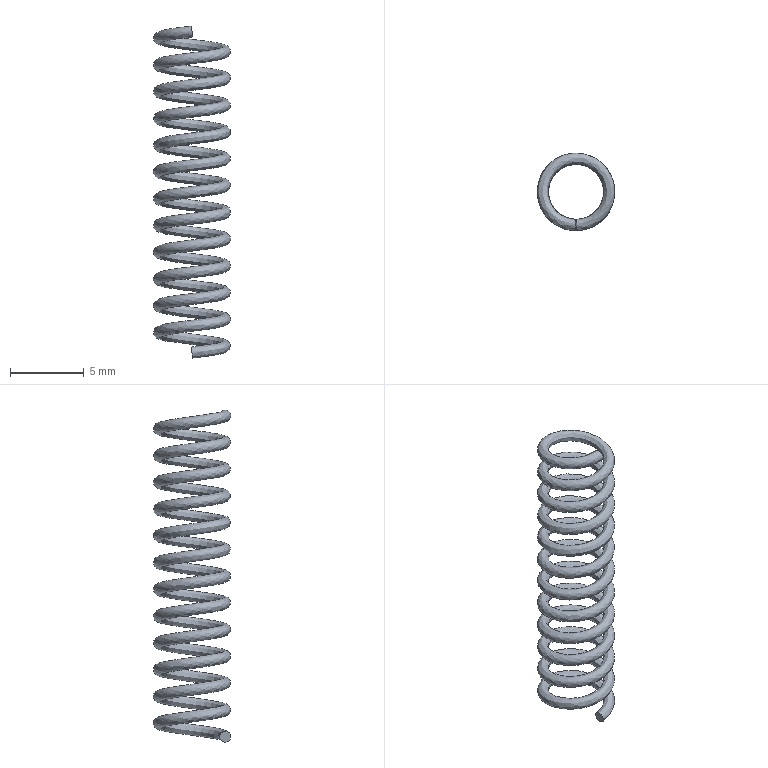Part | STEP file | 1-03.3 | 1 solid | 3 faces | box 5.252 x 5.25 x 22.544 mm | volume 75.49 mm3 | plane 2 | spline 1